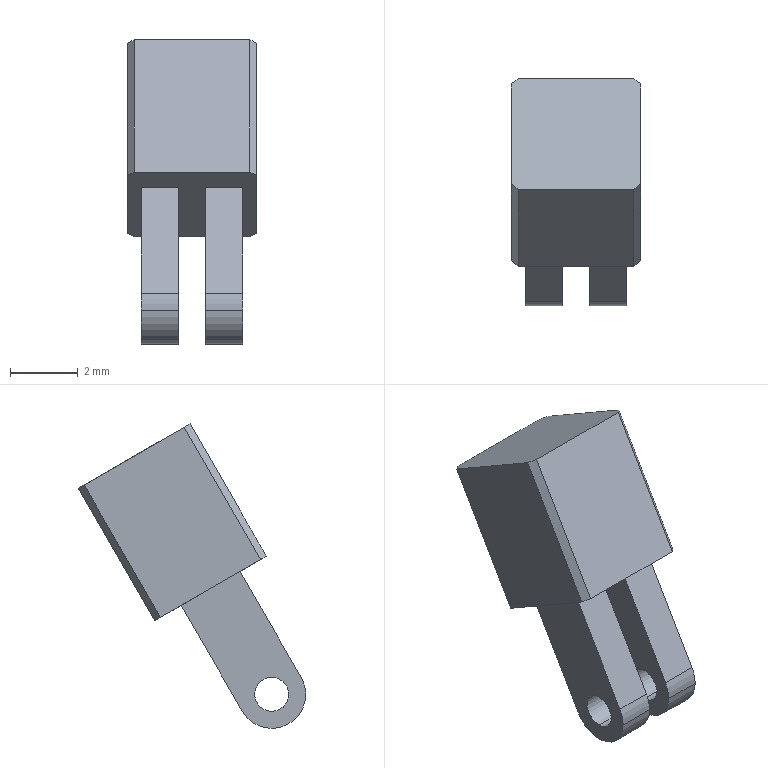Part | STEP file | 05-01 bending press head | 1 solid | 28 faces | box 3.8 x 6.694 x 8.962 mm | volume 82.141 mm3 | plane 18 | cylinder 10 | commonest cylinder face diameters 2 x6 1 x4
STEP:
#1=CARTESIAN_POINT('',(-6.355,-32.6,-2.678));
#2=VERTEX_POINT('',#1);
#3=CARTESIAN_POINT('',(-6.355,-32.1,-3.544));
#4=VERTEX_POINT('',#3);
#5=CARTESIAN_POINT('',(-6.355,-31.6,-2.678));
#6=DIRECTION('',(1.,0.,0.));
#7=DIRECTION('',(0.,0.,1.));
#8=AXIS2_PLACEMENT_3D('',#5,#6,#7);
#9=CIRCLE('',#8,1.);
#10=EDGE_CURVE('',#2,#4,#9,.T.);
#11=ORIENTED_EDGE('',*,*,#10,.F.);
#12=CARTESIAN_POINT('',(-7.455,-32.6,-2.678));
#13=VERTEX_POINT('',#12);
#14=CARTESIAN_POINT('',(-14.455,-32.6,-2.678));
#15=DIRECTION('',(-1.,0.,0.));
#16=VECTOR('',#15,1000.);
#17=LINE('',#14,#16);
#18=EDGE_CURVE('',#2,#13,#17,.T.);
#19=ORIENTED_EDGE('',*,*,#18,.T.);
#20=CARTESIAN_POINT('',(-7.455,-32.1,-3.544));
#21=VERTEX_POINT('',#20);
#22=CARTESIAN_POINT('',(-7.455,-31.6,-2.678));
#23=DIRECTION('',(-1.,0.,0.));
#24=DIRECTION('',(0.,0.,-1.));
#25=AXIS2_PLACEMENT_3D('',#22,#23,#24);
#26=CIRCLE('',#25,1.);
#27=EDGE_CURVE('',#21,#13,#26,.T.);
#28=ORIENTED_EDGE('',*,*,#27,.F.);
#29=CARTESIAN_POINT('',(-6.355,-32.1,-3.544));
#30=DIRECTION('',(1.,0.,0.));
#31=VECTOR('',#30,1000.);
#32=LINE('',#29,#31);
#33=EDGE_CURVE('',#21,#4,#32,.T.);
#34=ORIENTED_EDGE('',*,*,#33,.T.);
#35=EDGE_LOOP('',(#11,#19,#28,#34));
#36=FACE_OUTER_BOUND('',#35,.T.);
#37=CARTESIAN_POINT('',(-14.455,-31.6,-2.678));
#38=DIRECTION('',(-1.,0.,0.));
#39=DIRECTION('',(0.,-1.,0.));
#40=AXIS2_PLACEMENT_3D('',#37,#38,#39);
#41=CYLINDRICAL_SURFACE('',#40,1.);
#42=ADVANCED_FACE('',(#36),#41,.T.);
#43=CARTESIAN_POINT('',(-4.455,-32.6,-2.678));
#44=VERTEX_POINT('',#43);
#45=CARTESIAN_POINT('',(-4.455,-32.1,-3.544));
#46=VERTEX_POINT('',#45);
#47=CARTESIAN_POINT('',(-4.455,-31.6,-2.678));
#48=DIRECTION('',(1.,0.,0.));
#49=DIRECTION('',(0.,0.,1.));
#50=AXIS2_PLACEMENT_3D('',#47,#48,#49);
#51=CIRCLE('',#50,1.);
#52=EDGE_CURVE('',#44,#46,#51,.T.);
#53=ORIENTED_EDGE('',*,*,#52,.F.);
#54=CARTESIAN_POINT('',(-5.555,-32.6,-2.678));
#55=VERTEX_POINT('',#54);
#56=CARTESIAN_POINT('',(-14.455,-32.6,-2.678));
#57=DIRECTION('',(-1.,0.,0.));
#58=VECTOR('',#57,1000.);
#59=LINE('',#56,#58);
#60=EDGE_CURVE('',#44,#55,#59,.T.);
#61=ORIENTED_EDGE('',*,*,#60,.T.);
#62=CARTESIAN_POINT('',(-5.555,-32.1,-3.544));
#63=VERTEX_POINT('',#62);
#64=CARTESIAN_POINT('',(-5.555,-31.6,-2.678));
#65=DIRECTION('',(-1.,0.,0.));
#66=DIRECTION('',(0.,0.,-1.));
#67=AXIS2_PLACEMENT_3D('',#64,#65,#66);
#68=CIRCLE('',#67,1.);
#69=EDGE_CURVE('',#63,#55,#68,.T.);
#70=ORIENTED_EDGE('',*,*,#69,.F.);
#71=CARTESIAN_POINT('',(-4.455,-32.1,-3.544));
#72=DIRECTION('',(1.,0.,0.));
#73=VECTOR('',#72,1000.);
#74=LINE('',#71,#73);
#75=EDGE_CURVE('',#63,#46,#74,.T.);
#76=ORIENTED_EDGE('',*,*,#75,.T.);
#77=EDGE_LOOP('',(#53,#61,#70,#76));
#78=FACE_OUTER_BOUND('',#77,.T.);
#79=CARTESIAN_POINT('',(-14.455,-31.6,-2.678));
#80=DIRECTION('',(-1.,0.,0.));
#81=DIRECTION('',(0.,-1.,0.));
#82=AXIS2_PLACEMENT_3D('',#79,#80,#81);
#83=CYLINDRICAL_SURFACE('',#82,1.);
#84=ADVANCED_FACE('',(#78),#83,.T.);
#85=CARTESIAN_POINT('',(-6.355,-31.6,-3.178));
#86=VERTEX_POINT('',#85);
#87=CARTESIAN_POINT('',(-6.355,-31.6,-2.178));
#88=VERTEX_POINT('',#87);
#89=CARTESIAN_POINT('',(-6.355,-31.6,-2.678));
#90=DIRECTION('',(-1.,0.,0.));
#91=DIRECTION('',(0.,0.,1.));
#92=AXIS2_PLACEMENT_3D('',#89,#90,#91);
#93=CIRCLE('',#92,0.5);
#94=EDGE_CURVE('',#86,#88,#93,.T.);
#95=ORIENTED_EDGE('',*,*,#94,.F.);
#96=CARTESIAN_POINT('',(-7.455,-31.6,-3.178));
#97=VERTEX_POINT('',#96);
#98=CARTESIAN_POINT('',(2.545,-31.6,-3.178));
#99=DIRECTION('',(-1.,0.,0.));
#100=VECTOR('',#99,1000.);
#101=LINE('',#98,#100);
#102=EDGE_CURVE('',#86,#97,#101,.T.);
#103=ORIENTED_EDGE('',*,*,#102,.T.);
#104=CARTESIAN_POINT('',(-7.455,-31.6,-2.178));
#105=VERTEX_POINT('',#104);
#106=CARTESIAN_POINT('',(-7.455,-31.6,-2.678));
#107=DIRECTION('',(-1.,0.,0.));
#108=DIRECTION('',(0.,0.,1.));
#109=AXIS2_PLACEMENT_3D('',#106,#107,#108);
#110=CIRCLE('',#109,0.5);
#111=EDGE_CURVE('',#97,#105,#110,.T.);
#112=ORIENTED_EDGE('',*,*,#111,.T.);
#113=CARTESIAN_POINT('',(2.545,-31.6,-2.178));
#114=DIRECTION('',(-1.,0.,0.));
#115=VECTOR('',#114,1000.);
#116=LINE('',#113,#115);
#117=EDGE_CURVE('',#88,#105,#116,.T.);
#118=ORIENTED_EDGE('',*,*,#117,.F.);
#119=EDGE_LOOP('',(#95,#103,#112,#118));
#120=FACE_OUTER_BOUND('',#119,.T.);
#121=CARTESIAN_POINT('',(2.545,-31.6,-2.678));
#122=DIRECTION('',(-1.,0.,0.));
#123=DIRECTION('',(0.,0.,1.));
#124=AXIS2_PLACEMENT_3D('',#121,#122,#123);
#125=CYLINDRICAL_SURFACE('',#124,0.5);
#126=ADVANCED_FACE('',(#120),#125,.F.);
#127=CARTESIAN_POINT('',(-4.455,-31.6,-3.178));
#128=VERTEX_POINT('',#127);
#129=CARTESIAN_POINT('',(-4.455,-31.6,-2.178));
#130=VERTEX_POINT('',#129);
#131=CARTESIAN_POINT('',(-4.455,-31.6,-2.678));
#132=DIRECTION('',(-1.,0.,0.));
#133=DIRECTION('',(0.,0.,1.));
#134=AXIS2_PLACEMENT_3D('',#131,#132,#133);
#135=CIRCLE('',#134,0.5);
#136=EDGE_CURVE('',#128,#130,#135,.T.);
#137=ORIENTED_EDGE('',*,*,#136,.F.);
#138=CARTESIAN_POINT('',(-5.555,-31.6,-3.178));
#139=VERTEX_POINT('',#138);
#140=CARTESIAN_POINT('',(2.545,-31.6,-3.178));
#141=DIRECTION('',(-1.,0.,0.));
#142=VECTOR('',#141,1000.);
#143=LINE('',#140,#142);
#144=EDGE_CURVE('',#128,#139,#143,.T.);
#145=ORIENTED_EDGE('',*,*,#144,.T.);
#146=CARTESIAN_POINT('',(-5.555,-31.6,-2.178));
#147=VERTEX_POINT('',#146);
#148=CARTESIAN_POINT('',(-5.555,-31.6,-2.678));
#149=DIRECTION('',(1.,0.,0.));
#150=DIRECTION('',(0.,0.,-1.));
#151=AXIS2_PLACEMENT_3D('',#148,#149,#150);
#152=CIRCLE('',#151,0.5);
#153=EDGE_CURVE('',#147,#139,#152,.T.);
#154=ORIENTED_EDGE('',*,*,#153,.F.);
#155=CARTESIAN_POINT('',(2.545,-31.6,-2.178));
#156=DIRECTION('',(-1.,0.,0.));
#157=VECTOR('',#156,1000.);
#158=LINE('',#155,#157);
#159=EDGE_CURVE('',#130,#147,#158,.T.);
#160=ORIENTED_EDGE('',*,*,#159,.F.);
#161=EDGE_LOOP('',(#137,#145,#154,#160));
#162=FACE_OUTER_BOUND('',#161,.T.);
#163=CARTESIAN_POINT('',(2.545,-31.6,-2.678));
#164=DIRECTION('',(-1.,0.,0.));
#165=DIRECTION('',(0.,0.,1.));
#166=AXIS2_PLACEMENT_3D('',#163,#164,#165);
#167=CYLINDRICAL_SURFACE('',#166,0.5);
#168=ADVANCED_FACE('',(#162),#167,.F.);
#169=CARTESIAN_POINT('',(-7.455,-32.466,-2.178));
#170=VERTEX_POINT('',#169);
#171=CARTESIAN_POINT('',(-7.455,-30.666,0.94));
#172=VERTEX_POINT('',#171);
#173=CARTESIAN_POINT('',(-7.455,-33.117,-3.305));
#174=DIRECTION('',(0.,0.5,0.866));
#175=VECTOR('',#174,1000.);
#176=LINE('',#173,#175);
#177=EDGE_CURVE('',#170,#172,#176,.T.);
#178=ORIENTED_EDGE('',*,*,#177,.F.);
#179=CARTESIAN_POINT('',(-6.355,-32.466,-2.178));
#180=VERTEX_POINT('',#179);
#181=CARTESIAN_POINT('',(-6.355,-32.466,-2.178));
#182=DIRECTION('',(1.,0.,0.));
#183=VECTOR('',#182,1000.);
#184=LINE('',#181,#183);
#185=EDGE_CURVE('',#170,#180,#184,.T.);
#186=ORIENTED_EDGE('',*,*,#185,.T.);
#187=CARTESIAN_POINT('',(-6.355,-30.666,0.94));
#188=VERTEX_POINT('',#187);
#189=CARTESIAN_POINT('',(-6.355,-31.166,0.074));
#190=DIRECTION('',(0.,-0.5,-0.866));
#191=VECTOR('',#190,1000.);
#192=LINE('',#189,#191);
#193=EDGE_CURVE('',#188,#180,#192,.T.);
#194=ORIENTED_EDGE('',*,*,#193,.F.);
#195=CARTESIAN_POINT('',(-14.455,-30.666,0.94));
#196=DIRECTION('',(1.,0.,0.));
#197=VECTOR('',#196,1000.);
#198=LINE('',#195,#197);
#199=EDGE_CURVE('',#172,#188,#198,.T.);
#200=ORIENTED_EDGE('',*,*,#199,.F.);
#201=EDGE_LOOP('',(#178,#186,#194,#200));
#202=FACE_OUTER_BOUND('',#201,.T.);
#203=CARTESIAN_POINT('',(-14.455,-31.166,0.074));
#204=DIRECTION('',(0.,0.866,-0.5));
#205=DIRECTION('',(0.,0.5,0.866));
#206=AXIS2_PLACEMENT_3D('',#203,#204,#205);
#207=PLANE('',#206);
#208=ADVANCED_FACE('',(#202),#207,.F.);
#209=CARTESIAN_POINT('',(-6.355,-28.934,-0.05998));
#210=VERTEX_POINT('',#209);
#211=CARTESIAN_POINT('',(-6.355,-30.734,-3.178));
#212=VERTEX_POINT('',#211);
#213=CARTESIAN_POINT('',(-6.355,-29.434,-0.926));
#214=DIRECTION('',(0.,-0.5,-0.866));
#215=VECTOR('',#214,1000.);
#216=LINE('',#213,#215);
#217=EDGE_CURVE('',#210,#212,#216,.T.);
#218=ORIENTED_EDGE('',*,*,#217,.T.);
#219=CARTESIAN_POINT('',(-7.455,-30.734,-3.178));
#220=VERTEX_POINT('',#219);
#221=CARTESIAN_POINT('',(-7.455,-30.734,-3.178));
#222=DIRECTION('',(-1.,0.,0.));
#223=VECTOR('',#222,1000.);
#224=LINE('',#221,#223);
#225=EDGE_CURVE('',#212,#220,#224,.T.);
#226=ORIENTED_EDGE('',*,*,#225,.T.);
#227=CARTESIAN_POINT('',(-7.455,-28.934,-0.05998));
#228=VERTEX_POINT('',#227);
#229=CARTESIAN_POINT('',(-7.455,-31.385,-4.305));
#230=DIRECTION('',(0.,-0.5,-0.866));
#231=VECTOR('',#230,1000.);
#232=LINE('',#229,#231);
#233=EDGE_CURVE('',#228,#220,#232,.T.);
#234=ORIENTED_EDGE('',*,*,#233,.F.);
#235=CARTESIAN_POINT('',(-4.455,-28.934,-0.05998));
#236=DIRECTION('',(1.,0.,0.));
#237=VECTOR('',#236,1000.);
#238=LINE('',#235,#237);
#239=EDGE_CURVE('',#228,#210,#238,.T.);
#240=ORIENTED_EDGE('',*,*,#239,.T.);
#241=EDGE_LOOP('',(#218,#226,#234,#240));
#242=FACE_OUTER_BOUND('',#241,.T.);
#243=CARTESIAN_POINT('',(-14.455,-29.434,-0.926));
#244=DIRECTION('',(0.,-0.866,0.5));
#245=DIRECTION('',(0.,-0.5,-0.866));
#246=AXIS2_PLACEMENT_3D('',#243,#244,#245);
#247=PLANE('',#246);
#248=ADVANCED_FACE('',(#242),#247,.F.);
#249=CARTESIAN_POINT('',(-7.655,-28.154,-0.51));
#250=VERTEX_POINT('',#249);
#251=CARTESIAN_POINT('',(-4.255,-28.154,-0.51));
#252=VERTEX_POINT('',#251);
#253=CARTESIAN_POINT('',(-7.855,-28.154,-0.51));
#254=DIRECTION('',(1.,0.,0.));
#255=VECTOR('',#254,1000.);
#256=LINE('',#253,#255);
#257=EDGE_CURVE('',#250,#252,#256,.T.);
#258=ORIENTED_EDGE('',*,*,#257,.F.);
#259=CARTESIAN_POINT('',(-7.655,-25.906,3.384));
#260=VERTEX_POINT('',#259);
#261=CARTESIAN_POINT('',(-7.655,-26.126,3.003));
#262=DIRECTION('',(0.,0.5,0.866));
#263=VECTOR('',#262,1000.);
#264=LINE('',#261,#263);
#265=EDGE_CURVE('',#250,#260,#264,.T.);
#266=ORIENTED_EDGE('',*,*,#265,.T.);
#267=CARTESIAN_POINT('',(-4.255,-25.906,3.384));
#268=VERTEX_POINT('',#267);
#269=CARTESIAN_POINT('',(-7.655,-25.906,3.384));
#270=DIRECTION('',(-1.,0.,0.));
#271=VECTOR('',#270,1000.);
#272=LINE('',#269,#271);
#273=EDGE_CURVE('',#268,#260,#272,.T.);
#274=ORIENTED_EDGE('',*,*,#273,.F.);
#275=CARTESIAN_POINT('',(-4.255,-28.654,-1.376));
#276=DIRECTION('',(0.,-0.5,-0.866));
#277=VECTOR('',#276,1000.);
#278=LINE('',#275,#277);
#279=EDGE_CURVE('',#268,#252,#278,.T.);
#280=ORIENTED_EDGE('',*,*,#279,.T.);
#281=EDGE_LOOP('',(#258,#266,#274,#280));
#282=FACE_OUTER_BOUND('',#281,.T.);
#283=CARTESIAN_POINT('',(-7.855,-30.454,-4.494));
#284=DIRECTION('',(0.,0.866,-0.5));
#285=DIRECTION('',(0.,0.5,0.866));
#286=AXIS2_PLACEMENT_3D('',#283,#284,#285);
#287=PLANE('',#286);
#288=ADVANCED_FACE('',(#282),#287,.T.);
#289=CARTESIAN_POINT('',(-4.255,-31.445,1.39));
#290=VERTEX_POINT('',#289);
#291=CARTESIAN_POINT('',(-7.655,-31.445,1.39));
#292=VERTEX_POINT('',#291);
#293=CARTESIAN_POINT('',(-7.855,-31.445,1.39));
#294=DIRECTION('',(-1.,0.,0.));
#295=VECTOR('',#294,1000.);
#296=LINE('',#293,#295);
#297=EDGE_CURVE('',#290,#292,#296,.T.);
#298=ORIENTED_EDGE('',*,*,#297,.F.);
#299=CARTESIAN_POINT('',(-4.255,-29.197,5.284));
#300=VERTEX_POINT('',#299);
#301=CARTESIAN_POINT('',(-4.255,-29.417,4.903));
#302=DIRECTION('',(0.,0.5,0.866));
#303=VECTOR('',#302,1000.);
#304=LINE('',#301,#303);
#305=EDGE_CURVE('',#290,#300,#304,.T.);
#306=ORIENTED_EDGE('',*,*,#305,.T.);
#307=CARTESIAN_POINT('',(-7.655,-29.197,5.284));
#308=VERTEX_POINT('',#307);
#309=CARTESIAN_POINT('',(-7.655,-29.197,5.284));
#310=DIRECTION('',(1.,0.,0.));
#311=VECTOR('',#310,1000.);
#312=LINE('',#309,#311);
#313=EDGE_CURVE('',#308,#300,#312,.T.);
#314=ORIENTED_EDGE('',*,*,#313,.F.);
#315=CARTESIAN_POINT('',(-7.655,-31.945,0.524));
#316=DIRECTION('',(0.,-0.5,-0.866));
#317=VECTOR('',#316,1000.);
#318=LINE('',#315,#317);
#319=EDGE_CURVE('',#308,#292,#318,.T.);
#320=ORIENTED_EDGE('',*,*,#319,.T.);
#321=EDGE_LOOP('',(#298,#306,#314,#320));
#322=FACE_OUTER_BOUND('',#321,.T.);
#323=CARTESIAN_POINT('',(-7.855,-29.417,4.903));
#324=DIRECTION('',(0.,-0.866,0.5));
#325=DIRECTION('',(0.,-0.5,-0.866));
#326=AXIS2_PLACEMENT_3D('',#323,#324,#325);
#327=PLANE('',#326);
#328=ADVANCED_FACE('',(#322),#327,.T.);
#329=CARTESIAN_POINT('',(-7.855,-28.327,-0.41));
#330=VERTEX_POINT('',#329);
#331=CARTESIAN_POINT('',(-7.855,-31.272,1.29));
#332=VERTEX_POINT('',#331);
#333=CARTESIAN_POINT('',(-7.855,-31.445,1.39));
#334=DIRECTION('',(0.,-0.866,0.5));
#335=VECTOR('',#334,1000.);
#336=LINE('',#333,#335);
#337=EDGE_CURVE('',#330,#332,#336,.T.);
#338=ORIENTED_EDGE('',*,*,#337,.T.);
#339=CARTESIAN_POINT('',(-7.855,-29.024,5.184));
#340=VERTEX_POINT('',#339);
#341=CARTESIAN_POINT('',(-7.855,-29.244,4.803));
#342=DIRECTION('',(0.,0.5,0.866));
#343=VECTOR('',#342,1000.);
#344=LINE('',#341,#343);
#345=EDGE_CURVE('',#332,#340,#344,.T.);
#346=ORIENTED_EDGE('',*,*,#345,.T.);
#347=CARTESIAN_POINT('',(-7.855,-26.079,3.484));
#348=VERTEX_POINT('',#347);
#349=CARTESIAN_POINT('',(-7.855,-26.079,3.484));
#350=DIRECTION('',(0.,-0.866,0.5));
#351=VECTOR('',#350,1000.);
#352=LINE('',#349,#351);
#353=EDGE_CURVE('',#348,#340,#352,.T.);
#354=ORIENTED_EDGE('',*,*,#353,.F.);
#355=CARTESIAN_POINT('',(-7.855,-28.827,-1.276));
#356=DIRECTION('',(0.,-0.5,-0.866));
#357=VECTOR('',#356,1000.);
#358=LINE('',#355,#357);
#359=EDGE_CURVE('',#348,#330,#358,.T.);
#360=ORIENTED_EDGE('',*,*,#359,.T.);
#361=EDGE_LOOP('',(#338,#346,#354,#360));
#362=FACE_OUTER_BOUND('',#361,.T.);
#363=CARTESIAN_POINT('',(-7.855,-29.417,4.903));
#364=DIRECTION('',(1.,0.,0.));
#365=DIRECTION('',(0.,0.,-1.));
#366=AXIS2_PLACEMENT_3D('',#363,#364,#365);
#367=PLANE('',#366);
#368=ADVANCED_FACE('',(#362),#367,.F.);
#369=CARTESIAN_POINT('',(-4.055,-28.327,-0.41));
#370=VERTEX_POINT('',#369);
#371=CARTESIAN_POINT('',(-4.055,-26.079,3.484));
#372=VERTEX_POINT('',#371);
#373=CARTESIAN_POINT('',(-4.055,-26.299,3.103));
#374=DIRECTION('',(0.,0.5,0.866));
#375=VECTOR('',#374,1000.);
#376=LINE('',#373,#375);
#377=EDGE_CURVE('',#370,#372,#376,.T.);
#378=ORIENTED_EDGE('',*,*,#377,.T.);
#379=CARTESIAN_POINT('',(-4.055,-29.024,5.184));
#380=VERTEX_POINT('',#379);
#381=CARTESIAN_POINT('',(-4.055,-26.079,3.484));
#382=DIRECTION('',(0.,0.866,-0.5));
#383=VECTOR('',#382,1000.);
#384=LINE('',#381,#383);
#385=EDGE_CURVE('',#380,#372,#384,.T.);
#386=ORIENTED_EDGE('',*,*,#385,.F.);
#387=CARTESIAN_POINT('',(-4.055,-31.272,1.29));
#388=VERTEX_POINT('',#387);
#389=CARTESIAN_POINT('',(-4.055,-31.772,0.424));
#390=DIRECTION('',(0.,-0.5,-0.866));
#391=VECTOR('',#390,1000.);
#392=LINE('',#389,#391);
#393=EDGE_CURVE('',#380,#388,#392,.T.);
#394=ORIENTED_EDGE('',*,*,#393,.T.);
#395=CARTESIAN_POINT('',(-4.055,-28.154,-0.51));
#396=DIRECTION('',(0.,0.866,-0.5));
#397=VECTOR('',#396,1000.);
#398=LINE('',#395,#397);
#399=EDGE_CURVE('',#388,#370,#398,.T.);
#400=ORIENTED_EDGE('',*,*,#399,.T.);
#401=EDGE_LOOP('',(#378,#386,#394,#400));
#402=FACE_OUTER_BOUND('',#401,.T.);
#403=CARTESIAN_POINT('',(-4.055,-26.126,3.003));
#404=DIRECTION('',(-1.,0.,0.));
#405=DIRECTION('',(0.,0.,1.));
#406=AXIS2_PLACEMENT_3D('',#403,#404,#405);
#407=PLANE('',#406);
#408=ADVANCED_FACE('',(#402),#407,.F.);
#409=CARTESIAN_POINT('',(-4.455,-31.6,-2.678));
#410=DIRECTION('',(-1.,0.,0.));
#411=DIRECTION('',(0.,0.,1.));
#412=AXIS2_PLACEMENT_3D('',#409,#410,#411);
#413=CIRCLE('',#412,0.5);
#414=EDGE_CURVE('',#130,#128,#413,.T.);
#415=ORIENTED_EDGE('',*,*,#414,.T.);
#416=ORIENTED_EDGE('',*,*,#136,.T.);
#417=EDGE_LOOP('',(#415,#416));
#418=FACE_BOUND('',#417,.T.);
#419=CARTESIAN_POINT('',(-4.455,-32.466,-2.178));
#420=VERTEX_POINT('',#419);
#421=CARTESIAN_POINT('',(-4.455,-30.666,0.94));
#422=VERTEX_POINT('',#421);
#423=CARTESIAN_POINT('',(-4.455,-31.166,0.074));
#424=DIRECTION('',(0.,0.5,0.866));
#425=VECTOR('',#424,1000.);
#426=LINE('',#423,#425);
#427=EDGE_CURVE('',#420,#422,#426,.T.);
#428=ORIENTED_EDGE('',*,*,#427,.F.);
#429=CARTESIAN_POINT('',(-4.455,-31.6,-2.678));
#430=DIRECTION('',(1.,0.,0.));
#431=DIRECTION('',(0.,0.,1.));
#432=AXIS2_PLACEMENT_3D('',#429,#430,#431);
#433=CIRCLE('',#432,1.);
#434=EDGE_CURVE('',#420,#44,#433,.T.);
#435=ORIENTED_EDGE('',*,*,#434,.T.);
#436=ORIENTED_EDGE('',*,*,#52,.T.);
#437=CARTESIAN_POINT('',(-4.455,-30.734,-3.178));
#438=VERTEX_POINT('',#437);
#439=CARTESIAN_POINT('',(-4.455,-31.6,-2.678));
#440=DIRECTION('',(1.,0.,0.));
#441=DIRECTION('',(0.,0.,1.));
#442=AXIS2_PLACEMENT_3D('',#439,#440,#441);
#443=CIRCLE('',#442,1.);
#444=EDGE_CURVE('',#46,#438,#443,.T.);
#445=ORIENTED_EDGE('',*,*,#444,.T.);
#446=CARTESIAN_POINT('',(-4.455,-28.934,-0.05998));
#447=VERTEX_POINT('',#446);
#448=CARTESIAN_POINT('',(-4.455,-29.434,-0.926));
#449=DIRECTION('',(0.,-0.5,-0.866));
#450=VECTOR('',#449,1000.);
#451=LINE('',#448,#450);
#452=EDGE_CURVE('',#447,#438,#451,.T.);
#453=ORIENTED_EDGE('',*,*,#452,.F.);
#454=CARTESIAN_POINT('',(-4.455,-36.814,4.49));
#455=DIRECTION('',(0.,0.866,-0.5));
#456=VECTOR('',#455,1000.);
#457=LINE('',#454,#456);
#458=EDGE_CURVE('',#422,#447,#457,.T.);
#459=ORIENTED_EDGE('',*,*,#458,.F.);
#460=EDGE_LOOP('',(#428,#435,#436,#445,#453,#459));
#461=FACE_OUTER_BOUND('',#460,.T.);
#462=CARTESIAN_POINT('',(-4.455,-39.265,0.2448));
#463=DIRECTION('',(-1.,0.,0.));
#464=DIRECTION('',(0.,0.,1.));
#465=AXIS2_PLACEMENT_3D('',#462,#463,#464);
#466=PLANE('',#465);
#467=ADVANCED_FACE('',(#418,#461),#466,.F.);
#468=CARTESIAN_POINT('',(-6.355,-36.814,4.49));
#469=DIRECTION('',(0.,-0.866,0.5));
#470=VECTOR('',#469,1000.);
#471=LINE('',#468,#470);
#472=EDGE_CURVE('',#210,#188,#471,.T.);
#473=ORIENTED_EDGE('',*,*,#472,.F.);
#474=ORIENTED_EDGE('',*,*,#239,.F.);
#475=CARTESIAN_POINT('',(-7.455,-36.814,4.49));
#476=DIRECTION('',(0.,0.866,-0.5));
#477=VECTOR('',#476,1000.);
#478=LINE('',#475,#477);
#479=EDGE_CURVE('',#172,#228,#478,.T.);
#480=ORIENTED_EDGE('',*,*,#479,.F.);
#481=ORIENTED_EDGE('',*,*,#199,.T.);
#482=EDGE_LOOP('',(#473,#474,#480,#481));
#483=FACE_BOUND('',#482,.T.);
#484=ORIENTED_EDGE('',*,*,#399,.F.);
#485=CARTESIAN_POINT('',(-4.055,-31.272,1.29));
#486=DIRECTION('',(-0.7071,-0.6124,0.3536));
#487=VECTOR('',#486,1000.);
#488=LINE('',#485,#487);
#489=EDGE_CURVE('',#388,#290,#488,.T.);
#490=ORIENTED_EDGE('',*,*,#489,.T.);
#491=ORIENTED_EDGE('',*,*,#297,.T.);
#492=CARTESIAN_POINT('',(-7.655,-31.445,1.39));
#493=DIRECTION('',(-0.7071,0.6124,-0.3536));
#494=VECTOR('',#493,1000.);
#495=LINE('',#492,#494);
#496=EDGE_CURVE('',#292,#332,#495,.T.);
#497=ORIENTED_EDGE('',*,*,#496,.T.);
#498=ORIENTED_EDGE('',*,*,#337,.F.);
#499=CARTESIAN_POINT('',(-7.655,-28.154,-0.51));
#500=DIRECTION('',(0.7071,0.6124,-0.3536));
#501=VECTOR('',#500,1000.);
#502=LINE('',#499,#501);
#503=EDGE_CURVE('',#330,#250,#502,.T.);
#504=ORIENTED_EDGE('',*,*,#503,.T.);
#505=ORIENTED_EDGE('',*,*,#257,.T.);
#506=CARTESIAN_POINT('',(-4.055,-28.327,-0.41));
#507=DIRECTION('',(0.7071,-0.6124,0.3536));
#508=VECTOR('',#507,1000.);
#509=LINE('',#506,#508);
#510=EDGE_CURVE('',#252,#370,#509,.T.);
#511=ORIENTED_EDGE('',*,*,#510,.T.);
#512=EDGE_LOOP('',(#484,#490,#491,#497,#498,#504,#505,#511));
#513=FACE_OUTER_BOUND('',#512,.T.);
#514=CARTESIAN_POINT('',(-5.555,-28.934,-0.05998));
#515=VERTEX_POINT('',#514);
#516=CARTESIAN_POINT('',(-4.455,-28.934,-0.05998));
#517=DIRECTION('',(1.,0.,0.));
#518=VECTOR('',#517,1000.);
#519=LINE('',#516,#518);
#520=EDGE_CURVE('',#515,#447,#519,.T.);
#521=ORIENTED_EDGE('',*,*,#520,.F.);
#522=CARTESIAN_POINT('',(-5.555,-30.666,0.94));
#523=VERTEX_POINT('',#522);
#524=CARTESIAN_POINT('',(-5.555,-22.005,-4.06));
#525=DIRECTION('',(0.,-0.866,0.5));
#526=VECTOR('',#525,1000.);
#527=LINE('',#524,#526);
#528=EDGE_CURVE('',#515,#523,#527,.T.);
#529=ORIENTED_EDGE('',*,*,#528,.T.);
#530=CARTESIAN_POINT('',(-14.455,-30.666,0.94));
#531=DIRECTION('',(1.,0.,0.));
#532=VECTOR('',#531,1000.);
#533=LINE('',#530,#532);
#534=EDGE_CURVE('',#523,#422,#533,.T.);
#535=ORIENTED_EDGE('',*,*,#534,.T.);
#536=ORIENTED_EDGE('',*,*,#458,.T.);
#537=EDGE_LOOP('',(#521,#529,#535,#536));
#538=FACE_BOUND('',#537,.T.);
#539=CARTESIAN_POINT('',(-4.455,-36.814,4.49));
#540=DIRECTION('',(0.,0.5,0.866));
#541=DIRECTION('',(0.,-0.866,0.5));
#542=AXIS2_PLACEMENT_3D('',#539,#540,#541);
#543=PLANE('',#542);
#544=ADVANCED_FACE('',(#483,#513,#538),#543,.F.);
#545=CARTESIAN_POINT('',(-7.455,-31.6,-2.678));
#546=DIRECTION('',(-1.,0.,0.));
#547=DIRECTION('',(0.,0.,1.));
#548=AXIS2_PLACEMENT_3D('',#545,#546,#547);
#549=CIRCLE('',#548,0.5);
#550=EDGE_CURVE('',#105,#97,#549,.T.);
#551=ORIENTED_EDGE('',*,*,#550,.F.);
#552=ORIENTED_EDGE('',*,*,#111,.F.);
#553=EDGE_LOOP('',(#551,#552));
#554=FACE_BOUND('',#553,.T.);
#555=CARTESIAN_POINT('',(-7.455,-31.6,-2.678));
#556=DIRECTION('',(-1.,0.,0.));
#557=DIRECTION('',(0.,0.,-1.));
#558=AXIS2_PLACEMENT_3D('',#555,#556,#557);
#559=CIRCLE('',#558,1.);
#560=EDGE_CURVE('',#220,#21,#559,.T.);
#561=ORIENTED_EDGE('',*,*,#560,.T.);
#562=ORIENTED_EDGE('',*,*,#27,.T.);
#563=CARTESIAN_POINT('',(-7.455,-31.6,-2.678));
#564=DIRECTION('',(-1.,0.,0.));
#565=DIRECTION('',(0.,0.,-1.));
#566=AXIS2_PLACEMENT_3D('',#563,#564,#565);
#567=CIRCLE('',#566,1.);
#568=EDGE_CURVE('',#13,#170,#567,.T.);
#569=ORIENTED_EDGE('',*,*,#568,.T.);
#570=ORIENTED_EDGE('',*,*,#177,.T.);
#571=ORIENTED_EDGE('',*,*,#479,.T.);
#572=ORIENTED_EDGE('',*,*,#233,.T.);
#573=EDGE_LOOP('',(#561,#562,#569,#570,#571,#572));
#574=FACE_OUTER_BOUND('',#573,.T.);
#575=CARTESIAN_POINT('',(-7.455,-39.265,0.2448));
#576=DIRECTION('',(1.,0.,0.));
#577=DIRECTION('',(0.,0.,-1.));
#578=AXIS2_PLACEMENT_3D('',#575,#576,#577);
#579=PLANE('',#578);
#580=ADVANCED_FACE('',(#554,#574),#579,.F.);
#581=CARTESIAN_POINT('',(-5.555,-32.466,-2.178));
#582=VERTEX_POINT('',#581);
#583=CARTESIAN_POINT('',(-5.555,-31.166,0.074));
#584=DIRECTION('',(0.,0.5,0.866));
#585=VECTOR('',#584,1000.);
#586=LINE('',#583,#585);
#587=EDGE_CURVE('',#582,#523,#586,.T.);
#588=ORIENTED_EDGE('',*,*,#587,.F.);
#589=CARTESIAN_POINT('',(-4.455,-32.466,-2.178));
#590=DIRECTION('',(1.,0.,0.));
#591=VECTOR('',#590,1000.);
#592=LINE('',#589,#591);
#593=EDGE_CURVE('',#582,#420,#592,.T.);
#594=ORIENTED_EDGE('',*,*,#593,.T.);
#595=ORIENTED_EDGE('',*,*,#427,.T.);
#596=ORIENTED_EDGE('',*,*,#534,.F.);
#597=EDGE_LOOP('',(#588,#594,#595,#596));
#598=FACE_OUTER_BOUND('',#597,.T.);
#599=CARTESIAN_POINT('',(-14.455,-31.166,0.074));
#600=DIRECTION('',(0.,0.866,-0.5));
#601=DIRECTION('',(0.,0.5,0.866));
#602=AXIS2_PLACEMENT_3D('',#599,#600,#601);
#603=PLANE('',#602);
#604=ADVANCED_FACE('',(#598),#603,.F.);
#605=ORIENTED_EDGE('',*,*,#452,.T.);
#606=CARTESIAN_POINT('',(-5.555,-30.734,-3.178));
#607=VERTEX_POINT('',#606);
#608=CARTESIAN_POINT('',(-5.555,-30.734,-3.178));
#609=DIRECTION('',(-1.,0.,0.));
#610=VECTOR('',#609,1000.);
#611=LINE('',#608,#610);
#612=EDGE_CURVE('',#438,#607,#611,.T.);
#613=ORIENTED_EDGE('',*,*,#612,.T.);
#614=CARTESIAN_POINT('',(-5.555,-29.434,-0.926));
#615=DIRECTION('',(0.,0.5,0.866));
#616=VECTOR('',#615,1000.);
#617=LINE('',#614,#616);
#618=EDGE_CURVE('',#607,#515,#617,.T.);
#619=ORIENTED_EDGE('',*,*,#618,.T.);
#620=ORIENTED_EDGE('',*,*,#520,.T.);
#621=EDGE_LOOP('',(#605,#613,#619,#620));
#622=FACE_OUTER_BOUND('',#621,.T.);
#623=CARTESIAN_POINT('',(-14.455,-29.434,-0.926));
#624=DIRECTION('',(0.,-0.866,0.5));
#625=DIRECTION('',(0.,-0.5,-0.866));
#626=AXIS2_PLACEMENT_3D('',#623,#624,#625);
#627=PLANE('',#626);
#628=ADVANCED_FACE('',(#622),#627,.F.);
#629=CARTESIAN_POINT('',(-6.355,-31.6,-2.678));
#630=DIRECTION('',(-1.,0.,0.));
#631=DIRECTION('',(0.,0.,1.));
#632=AXIS2_PLACEMENT_3D('',#629,#630,#631);
#633=CIRCLE('',#632,0.5);
#634=EDGE_CURVE('',#88,#86,#633,.T.);
#635=ORIENTED_EDGE('',*,*,#634,.T.);
#636=ORIENTED_EDGE('',*,*,#94,.T.);
#637=EDGE_LOOP('',(#635,#636));
#638=FACE_BOUND('',#637,.T.);
#639=ORIENTED_EDGE('',*,*,#193,.T.);
#640=CARTESIAN_POINT('',(-6.355,-31.6,-2.678));
#641=DIRECTION('',(1.,0.,0.));
#642=DIRECTION('',(0.,0.,1.));
#643=AXIS2_PLACEMENT_3D('',#640,#641,#642);
#644=CIRCLE('',#643,1.);
#645=EDGE_CURVE('',#180,#2,#644,.T.);
#646=ORIENTED_EDGE('',*,*,#645,.T.);
#647=ORIENTED_EDGE('',*,*,#10,.T.);
#648=CARTESIAN_POINT('',(-6.355,-31.6,-2.678));
#649=DIRECTION('',(1.,0.,0.));
#650=DIRECTION('',(0.,0.,1.));
#651=AXIS2_PLACEMENT_3D('',#648,#649,#650);
#652=CIRCLE('',#651,1.);
#653=EDGE_CURVE('',#4,#212,#652,.T.);
#654=ORIENTED_EDGE('',*,*,#653,.T.);
#655=ORIENTED_EDGE('',*,*,#217,.F.);
#656=ORIENTED_EDGE('',*,*,#472,.T.);
#657=EDGE_LOOP('',(#639,#646,#647,#654,#655,#656));
#658=FACE_OUTER_BOUND('',#657,.T.);
#659=CARTESIAN_POINT('',(-6.355,-22.505,-4.926));
#660=DIRECTION('',(-1.,0.,0.));
#661=DIRECTION('',(0.,0.,1.));
#662=AXIS2_PLACEMENT_3D('',#659,#660,#661);
#663=PLANE('',#662);
#664=ADVANCED_FACE('',(#638,#658),#663,.F.);
#665=ORIENTED_EDGE('',*,*,#153,.T.);
#666=CARTESIAN_POINT('',(-5.555,-31.6,-2.678));
#667=DIRECTION('',(1.,0.,0.));
#668=DIRECTION('',(0.,0.,-1.));
#669=AXIS2_PLACEMENT_3D('',#666,#667,#668);
#670=CIRCLE('',#669,0.5);
#671=EDGE_CURVE('',#139,#147,#670,.T.);
#672=ORIENTED_EDGE('',*,*,#671,.T.);
#673=EDGE_LOOP('',(#665,#672));
#674=FACE_BOUND('',#673,.T.);
#675=CARTESIAN_POINT('',(-5.555,-31.6,-2.678));
#676=DIRECTION('',(-1.,0.,0.));
#677=DIRECTION('',(0.,0.,-1.));
#678=AXIS2_PLACEMENT_3D('',#675,#676,#677);
#679=CIRCLE('',#678,1.);
#680=EDGE_CURVE('',#607,#63,#679,.T.);
#681=ORIENTED_EDGE('',*,*,#680,.T.);
#682=ORIENTED_EDGE('',*,*,#69,.T.);
#683=CARTESIAN_POINT('',(-5.555,-31.6,-2.678));
#684=DIRECTION('',(-1.,0.,0.));
#685=DIRECTION('',(0.,0.,-1.));
#686=AXIS2_PLACEMENT_3D('',#683,#684,#685);
#687=CIRCLE('',#686,1.);
#688=EDGE_CURVE('',#55,#582,#687,.T.);
#689=ORIENTED_EDGE('',*,*,#688,.T.);
#690=ORIENTED_EDGE('',*,*,#587,.T.);
#691=ORIENTED_EDGE('',*,*,#528,.F.);
#692=ORIENTED_EDGE('',*,*,#618,.F.);
#693=EDGE_LOOP('',(#681,#682,#689,#690,#691,#692));
#694=FACE_OUTER_BOUND('',#693,.T.);
#695=CARTESIAN_POINT('',(-5.555,-22.505,-4.926));
#696=DIRECTION('',(1.,0.,0.));
#697=DIRECTION('',(0.,0.,-1.));
#698=AXIS2_PLACEMENT_3D('',#695,#696,#697);
#699=PLANE('',#698);
#700=ADVANCED_FACE('',(#674,#694),#699,.F.);
#701=ORIENTED_EDGE('',*,*,#144,.F.);
#702=ORIENTED_EDGE('',*,*,#414,.F.);
#703=ORIENTED_EDGE('',*,*,#159,.T.);
#704=ORIENTED_EDGE('',*,*,#671,.F.);
#705=EDGE_LOOP('',(#701,#702,#703,#704));
#706=FACE_OUTER_BOUND('',#705,.T.);
#707=CARTESIAN_POINT('',(2.545,-31.6,-2.678));
#708=DIRECTION('',(-1.,0.,0.));
#709=DIRECTION('',(0.,0.,1.));
#710=AXIS2_PLACEMENT_3D('',#707,#708,#709);
#711=CYLINDRICAL_SURFACE('',#710,0.5);
#712=ADVANCED_FACE('',(#706),#711,.F.);
#713=ORIENTED_EDGE('',*,*,#102,.F.);
#714=ORIENTED_EDGE('',*,*,#634,.F.);
#715=ORIENTED_EDGE('',*,*,#117,.T.);
#716=ORIENTED_EDGE('',*,*,#550,.T.);
#717=EDGE_LOOP('',(#713,#714,#715,#716));
#718=FACE_OUTER_BOUND('',#717,.T.);
#719=CARTESIAN_POINT('',(2.545,-31.6,-2.678));
#720=DIRECTION('',(-1.,0.,0.));
#721=DIRECTION('',(0.,0.,1.));
#722=AXIS2_PLACEMENT_3D('',#719,#720,#721);
#723=CYLINDRICAL_SURFACE('',#722,0.5);
#724=ADVANCED_FACE('',(#718),#723,.F.);
#725=ORIENTED_EDGE('',*,*,#393,.F.);
#726=CARTESIAN_POINT('',(-4.255,-29.197,5.284));
#727=DIRECTION('',(0.7071,0.6124,-0.3536));
#728=VECTOR('',#727,1000.);
#729=LINE('',#726,#728);
#730=EDGE_CURVE('',#300,#380,#729,.T.);
#731=ORIENTED_EDGE('',*,*,#730,.F.);
#732=ORIENTED_EDGE('',*,*,#305,.F.);
#733=ORIENTED_EDGE('',*,*,#489,.F.);
#734=EDGE_LOOP('',(#725,#731,#732,#733));
#735=FACE_OUTER_BOUND('',#734,.T.);
#736=CARTESIAN_POINT('',(-4.055,-29.244,4.803));
#737=DIRECTION('',(0.7071,-0.6124,0.3536));
#738=DIRECTION('',(0.6547,0.7559,0.));
#739=AXIS2_PLACEMENT_3D('',#736,#737,#738);
#740=PLANE('',#739);
#741=ADVANCED_FACE('',(#735),#740,.T.);
#742=ORIENTED_EDGE('',*,*,#319,.F.);
#743=CARTESIAN_POINT('',(-7.855,-29.024,5.184));
#744=DIRECTION('',(0.7071,-0.6124,0.3536));
#745=VECTOR('',#744,1000.);
#746=LINE('',#743,#745);
#747=EDGE_CURVE('',#340,#308,#746,.T.);
#748=ORIENTED_EDGE('',*,*,#747,.F.);
#749=ORIENTED_EDGE('',*,*,#345,.F.);
#750=ORIENTED_EDGE('',*,*,#496,.F.);
#751=EDGE_LOOP('',(#742,#748,#749,#750));
#752=FACE_OUTER_BOUND('',#751,.T.);
#753=CARTESIAN_POINT('',(-7.655,-29.417,4.903));
#754=DIRECTION('',(-0.7071,-0.6124,0.3536));
#755=DIRECTION('',(0.6547,-0.7559,0.));
#756=AXIS2_PLACEMENT_3D('',#753,#754,#755);
#757=PLANE('',#756);
#758=ADVANCED_FACE('',(#752),#757,.T.);
#759=ORIENTED_EDGE('',*,*,#503,.F.);
#760=ORIENTED_EDGE('',*,*,#359,.F.);
#761=CARTESIAN_POINT('',(-7.655,-25.906,3.384));
#762=DIRECTION('',(-0.7071,-0.6124,0.3536));
#763=VECTOR('',#762,1000.);
#764=LINE('',#761,#763);
#765=EDGE_CURVE('',#260,#348,#764,.T.);
#766=ORIENTED_EDGE('',*,*,#765,.F.);
#767=ORIENTED_EDGE('',*,*,#265,.F.);
#768=EDGE_LOOP('',(#759,#760,#766,#767));
#769=FACE_OUTER_BOUND('',#768,.T.);
#770=CARTESIAN_POINT('',(-7.655,-30.454,-4.494));
#771=DIRECTION('',(-0.7071,0.6124,-0.3536));
#772=DIRECTION('',(-0.6547,-0.7559,0.));
#773=AXIS2_PLACEMENT_3D('',#770,#771,#772);
#774=PLANE('',#773);
#775=ADVANCED_FACE('',(#769),#774,.T.);
#776=ORIENTED_EDGE('',*,*,#510,.F.);
#777=ORIENTED_EDGE('',*,*,#279,.F.);
#778=CARTESIAN_POINT('',(-4.055,-26.079,3.484));
#779=DIRECTION('',(-0.7071,0.6124,-0.3536));
#780=VECTOR('',#779,1000.);
#781=LINE('',#778,#780);
#782=EDGE_CURVE('',#372,#268,#781,.T.);
#783=ORIENTED_EDGE('',*,*,#782,.F.);
#784=ORIENTED_EDGE('',*,*,#377,.F.);
#785=EDGE_LOOP('',(#776,#777,#783,#784));
#786=FACE_OUTER_BOUND('',#785,.T.);
#787=CARTESIAN_POINT('',(-4.055,-26.299,3.103));
#788=DIRECTION('',(0.7071,0.6124,-0.3536));
#789=DIRECTION('',(-0.6547,0.7559,0.));
#790=AXIS2_PLACEMENT_3D('',#787,#788,#789);
#791=PLANE('',#790);
#792=ADVANCED_FACE('',(#786),#791,.T.);
#793=ORIENTED_EDGE('',*,*,#75,.F.);
#794=ORIENTED_EDGE('',*,*,#680,.F.);
#795=ORIENTED_EDGE('',*,*,#612,.F.);
#796=ORIENTED_EDGE('',*,*,#444,.F.);
#797=EDGE_LOOP('',(#793,#794,#795,#796));
#798=FACE_OUTER_BOUND('',#797,.T.);
#799=CARTESIAN_POINT('',(-14.455,-31.6,-2.678));
#800=DIRECTION('',(1.,0.,0.));
#801=DIRECTION('',(0.,1.,0.));
#802=AXIS2_PLACEMENT_3D('',#799,#800,#801);
#803=CYLINDRICAL_SURFACE('',#802,1.);
#804=ADVANCED_FACE('',(#798),#803,.T.);
#805=ORIENTED_EDGE('',*,*,#60,.F.);
#806=ORIENTED_EDGE('',*,*,#434,.F.);
#807=ORIENTED_EDGE('',*,*,#593,.F.);
#808=ORIENTED_EDGE('',*,*,#688,.F.);
#809=EDGE_LOOP('',(#805,#806,#807,#808));
#810=FACE_OUTER_BOUND('',#809,.T.);
#811=CARTESIAN_POINT('',(-14.455,-31.6,-2.678));
#812=DIRECTION('',(-1.,0.,0.));
#813=DIRECTION('',(0.,-1.,0.));
#814=AXIS2_PLACEMENT_3D('',#811,#812,#813);
#815=CYLINDRICAL_SURFACE('',#814,1.);
#816=ADVANCED_FACE('',(#810),#815,.T.);
#817=ORIENTED_EDGE('',*,*,#33,.F.);
#818=ORIENTED_EDGE('',*,*,#560,.F.);
#819=ORIENTED_EDGE('',*,*,#225,.F.);
#820=ORIENTED_EDGE('',*,*,#653,.F.);
#821=EDGE_LOOP('',(#817,#818,#819,#820));
#822=FACE_OUTER_BOUND('',#821,.T.);
#823=CARTESIAN_POINT('',(-14.455,-31.6,-2.678));
#824=DIRECTION('',(1.,0.,0.));
#825=DIRECTION('',(0.,1.,0.));
#826=AXIS2_PLACEMENT_3D('',#823,#824,#825);
#827=CYLINDRICAL_SURFACE('',#826,1.);
#828=ADVANCED_FACE('',(#822),#827,.T.);
#829=ORIENTED_EDGE('',*,*,#18,.F.);
#830=ORIENTED_EDGE('',*,*,#645,.F.);
#831=ORIENTED_EDGE('',*,*,#185,.F.);
#832=ORIENTED_EDGE('',*,*,#568,.F.);
#833=EDGE_LOOP('',(#829,#830,#831,#832));
#834=FACE_OUTER_BOUND('',#833,.T.);
#835=CARTESIAN_POINT('',(-14.455,-31.6,-2.678));
#836=DIRECTION('',(-1.,0.,0.));
#837=DIRECTION('',(0.,-1.,0.));
#838=AXIS2_PLACEMENT_3D('',#835,#836,#837);
#839=CYLINDRICAL_SURFACE('',#838,1.);
#840=ADVANCED_FACE('',(#834),#839,.T.);
#841=ORIENTED_EDGE('',*,*,#765,.T.);
#842=ORIENTED_EDGE('',*,*,#353,.T.);
#843=ORIENTED_EDGE('',*,*,#747,.T.);
#844=ORIENTED_EDGE('',*,*,#313,.T.);
#845=ORIENTED_EDGE('',*,*,#730,.T.);
#846=ORIENTED_EDGE('',*,*,#385,.T.);
#847=ORIENTED_EDGE('',*,*,#782,.T.);
#848=ORIENTED_EDGE('',*,*,#273,.T.);
#849=EDGE_LOOP('',(#841,#842,#843,#844,#845,#846,#847,#848));
#850=FACE_OUTER_BOUND('',#849,.T.);
#851=CARTESIAN_POINT('',(-9.555,-27.551,4.334));
#852=DIRECTION('',(0.,0.5,0.866));
#853=DIRECTION('',(0.,-0.866,0.5));
#854=AXIS2_PLACEMENT_3D('',#851,#852,#853);
#855=PLANE('',#854);
#856=ADVANCED_FACE('',(#850),#855,.T.);
#857=CLOSED_SHELL('',(#42,#84,#126,#168,#208,#248,#288,#328,#368,#408,#467,#544,#580,#604,#628,#664,#700,#712,#724,#741,#758,#775,#792,#804,#816,#828,#840,#856));
#858=MANIFOLD_SOLID_BREP('',#857);
#859=CARTESIAN_POINT('',(0.,0.,0.));
#860=DIRECTION('',(0.,0.,1.));
#861=DIRECTION('',(1.,0.,0.));
#862=AXIS2_PLACEMENT_3D('',#859,#860,#861);
#863=(LENGTH_UNIT()NAMED_UNIT(*)SI_UNIT(.MILLI.,.METRE.));
#864=UNCERTAINTY_MEASURE_WITH_UNIT(LENGTH_MEASURE(0.00001),#863,'','');
#865=(NAMED_UNIT(*)PLANE_ANGLE_UNIT()SI_UNIT($,.RADIAN.));
#866=(NAMED_UNIT(*)SI_UNIT($,.STERADIAN.)SOLID_ANGLE_UNIT());
#867=(GEOMETRIC_REPRESENTATION_CONTEXT(3)GLOBAL_UNCERTAINTY_ASSIGNED_CONTEXT((#864))GLOBAL_UNIT_ASSIGNED_CONTEXT((#863,#865,#866))REPRESENTATION_CONTEXT('',''));
#868=ADVANCED_BREP_SHAPE_REPRESENTATION('',(#858,#862),#867);